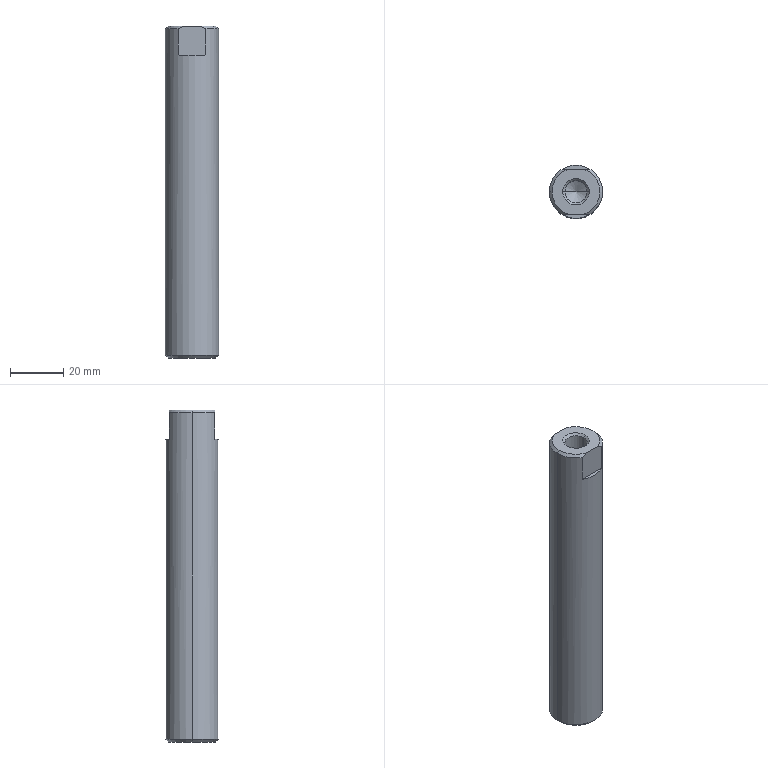Part | SolidWorks | features BaseBody 1 | 1 solid | 19 faces | box 20 x 20 x 125 mm | volume 37828 mm3 | cone 9 | plane 6 | cylinder 4 | commonest cylinder face diameters 8.376 x2 20 x2
STEP:
#1=CARTESIAN_POINT('',(10.,0.,-124.));
#2=VERTEX_POINT('',#1);
#3=CARTESIAN_POINT('',(-10.,0.,-124.));
#4=VERTEX_POINT('',#3);
#5=CARTESIAN_POINT('',(0.,0.,-124.));
#6=DIRECTION('',(0.,0.,1.));
#7=DIRECTION('',(1.,0.,0.));
#8=AXIS2_PLACEMENT_3D('',#5,#6,#7);
#9=CIRCLE('',#8,10.);
#10=EDGE_CURVE('',#2,#4,#9,.T.);
#11=ORIENTED_EDGE('',*,*,#10,.T.);
#12=CARTESIAN_POINT('',(-10.,0.,-1.));
#13=VERTEX_POINT('',#12);
#14=CARTESIAN_POINT('',(-10.,0.,-125.));
#15=DIRECTION('',(0.,0.,1.));
#16=VECTOR('',#15,1000.);
#17=LINE('',#14,#16);
#18=EDGE_CURVE('',#4,#13,#17,.T.);
#19=ORIENTED_EDGE('',*,*,#18,.T.);
#20=CARTESIAN_POINT('',(-5.268,8.5,-1.));
#21=VERTEX_POINT('',#20);
#22=CARTESIAN_POINT('',(0.,0.,-1.));
#23=DIRECTION('',(0.,0.,-1.));
#24=DIRECTION('',(1.,0.,0.));
#25=AXIS2_PLACEMENT_3D('',#22,#23,#24);
#26=CIRCLE('',#25,10.);
#27=EDGE_CURVE('',#13,#21,#26,.T.);
#28=ORIENTED_EDGE('',*,*,#27,.T.);
#29=CARTESIAN_POINT('',(-5.268,8.5,-11.));
#30=VERTEX_POINT('',#29);
#31=CARTESIAN_POINT('',(-5.268,8.5,-125.));
#32=DIRECTION('',(0.,0.,-1.));
#33=VECTOR('',#32,1000.);
#34=LINE('',#31,#33);
#35=EDGE_CURVE('',#21,#30,#34,.T.);
#36=ORIENTED_EDGE('',*,*,#35,.T.);
#37=CARTESIAN_POINT('',(5.268,8.5,-11.));
#38=VERTEX_POINT('',#37);
#39=CARTESIAN_POINT('',(0.,0.,-11.));
#40=DIRECTION('',(0.,0.,-1.));
#41=DIRECTION('',(1.,0.,0.));
#42=AXIS2_PLACEMENT_3D('',#39,#40,#41);
#43=CIRCLE('',#42,10.);
#44=EDGE_CURVE('',#30,#38,#43,.T.);
#45=ORIENTED_EDGE('',*,*,#44,.T.);
#46=CARTESIAN_POINT('',(5.268,8.5,-1.));
#47=VERTEX_POINT('',#46);
#48=CARTESIAN_POINT('',(5.268,8.5,-125.));
#49=DIRECTION('',(0.,0.,1.));
#50=VECTOR('',#49,1000.);
#51=LINE('',#48,#50);
#52=EDGE_CURVE('',#38,#47,#51,.T.);
#53=ORIENTED_EDGE('',*,*,#52,.T.);
#54=CARTESIAN_POINT('',(10.,0.,-1.));
#55=VERTEX_POINT('',#54);
#56=CARTESIAN_POINT('',(0.,0.,-1.));
#57=DIRECTION('',(0.,0.,-1.));
#58=DIRECTION('',(1.,0.,0.));
#59=AXIS2_PLACEMENT_3D('',#56,#57,#58);
#60=CIRCLE('',#59,10.);
#61=EDGE_CURVE('',#47,#55,#60,.T.);
#62=ORIENTED_EDGE('',*,*,#61,.T.);
#63=CARTESIAN_POINT('',(10.,0.,-125.));
#64=DIRECTION('',(0.,0.,1.));
#65=VECTOR('',#64,1000.);
#66=LINE('',#63,#65);
#67=EDGE_CURVE('',#2,#55,#66,.T.);
#68=ORIENTED_EDGE('',*,*,#67,.F.);
#69=EDGE_LOOP('',(#11,#19,#28,#36,#45,#53,#62,#68));
#70=FACE_OUTER_BOUND('',#69,.T.);
#71=CARTESIAN_POINT('',(0.,0.,-125.));
#72=DIRECTION('',(0.,0.,1.));
#73=DIRECTION('',(1.,0.,0.));
#74=AXIS2_PLACEMENT_3D('',#71,#72,#73);
#75=CYLINDRICAL_SURFACE('',#74,10.);
#76=ADVANCED_FACE('',(#70),#75,.T.);
#77=CARTESIAN_POINT('',(-2.958,-8.5,0.));
#78=VERTEX_POINT('',#77);
#79=CARTESIAN_POINT('',(-9.,0.,0.));
#80=VERTEX_POINT('',#79);
#81=CARTESIAN_POINT('',(0.,0.,0.));
#82=DIRECTION('',(0.,0.,-1.));
#83=DIRECTION('',(-1.,0.,0.));
#84=AXIS2_PLACEMENT_3D('',#81,#82,#83);
#85=CIRCLE('',#84,9.);
#86=EDGE_CURVE('',#78,#80,#85,.T.);
#87=ORIENTED_EDGE('',*,*,#86,.T.);
#88=CARTESIAN_POINT('',(-10.,0.,-1.));
#89=DIRECTION('',(-0.7071,0.,-0.7071));
#90=VECTOR('',#89,1000.);
#91=LINE('',#88,#90);
#92=EDGE_CURVE('',#80,#13,#91,.T.);
#93=ORIENTED_EDGE('',*,*,#92,.T.);
#94=CARTESIAN_POINT('',(-5.268,-8.5,-1.));
#95=VERTEX_POINT('',#94);
#96=CARTESIAN_POINT('',(0.,0.,-1.));
#97=DIRECTION('',(0.,0.,-1.));
#98=DIRECTION('',(1.,0.,0.));
#99=AXIS2_PLACEMENT_3D('',#96,#97,#98);
#100=CIRCLE('',#99,10.);
#101=EDGE_CURVE('',#95,#13,#100,.T.);
#102=ORIENTED_EDGE('',*,*,#101,.F.);
#103=CARTESIAN_POINT('',(-5.268,-8.5,-1.));
#104=CARTESIAN_POINT('',(-4.523,-8.5,-0.6078));
#105=CARTESIAN_POINT('',(-3.758,-8.5,-0.2631));
#106=CARTESIAN_POINT('',(-2.958,-8.5,0.));
#107=B_SPLINE_CURVE_WITH_KNOTS('',3,(#103,#104,#105,#106),.UNSPECIFIED.,.F.,.F.,(4,4),(0.,0.002517),.UNSPECIFIED.);
#108=EDGE_CURVE('',#95,#78,#107,.T.);
#109=ORIENTED_EDGE('',*,*,#108,.T.);
#110=EDGE_LOOP('',(#87,#93,#102,#109));
#111=FACE_OUTER_BOUND('',#110,.T.);
#112=CARTESIAN_POINT('',(0.,0.,-1.));
#113=DIRECTION('',(0.,0.,-1.));
#114=DIRECTION('',(-1.,0.,0.));
#115=AXIS2_PLACEMENT_3D('',#112,#113,#114);
#116=CONICAL_SURFACE('',#115,10.,0.7854);
#117=ADVANCED_FACE('',(#111),#116,.T.);
#118=CARTESIAN_POINT('',(9.,0.,-125.));
#119=VERTEX_POINT('',#118);
#120=CARTESIAN_POINT('',(-9.,0.,-125.));
#121=VERTEX_POINT('',#120);
#122=CARTESIAN_POINT('',(0.,0.,-125.));
#123=DIRECTION('',(0.,0.,1.));
#124=DIRECTION('',(1.,0.,0.));
#125=AXIS2_PLACEMENT_3D('',#122,#123,#124);
#126=CIRCLE('',#125,9.);
#127=EDGE_CURVE('',#119,#121,#126,.T.);
#128=ORIENTED_EDGE('',*,*,#127,.T.);
#129=CARTESIAN_POINT('',(-10.,0.,-124.));
#130=DIRECTION('',(-0.7071,0.,0.7071));
#131=VECTOR('',#130,1000.);
#132=LINE('',#129,#131);
#133=EDGE_CURVE('',#121,#4,#132,.T.);
#134=ORIENTED_EDGE('',*,*,#133,.T.);
#135=ORIENTED_EDGE('',*,*,#10,.F.);
#136=CARTESIAN_POINT('',(10.,0.,-124.));
#137=DIRECTION('',(0.7071,0.,0.7071));
#138=VECTOR('',#137,1000.);
#139=LINE('',#136,#138);
#140=EDGE_CURVE('',#119,#2,#139,.T.);
#141=ORIENTED_EDGE('',*,*,#140,.F.);
#142=EDGE_LOOP('',(#128,#134,#135,#141));
#143=FACE_OUTER_BOUND('',#142,.T.);
#144=CARTESIAN_POINT('',(0.,0.,-124.));
#145=DIRECTION('',(0.,0.,1.));
#146=DIRECTION('',(1.,0.,0.));
#147=AXIS2_PLACEMENT_3D('',#144,#145,#146);
#148=CONICAL_SURFACE('',#147,10.,0.7854);
#149=ADVANCED_FACE('',(#143),#148,.T.);
#150=CARTESIAN_POINT('',(-4.188,0.,-0.812));
#151=VERTEX_POINT('',#150);
#152=CARTESIAN_POINT('',(4.188,0.,-0.812));
#153=VERTEX_POINT('',#152);
#154=CARTESIAN_POINT('',(0.,0.,-0.812));
#155=DIRECTION('',(0.,0.,1.));
#156=DIRECTION('',(1.,0.,0.));
#157=AXIS2_PLACEMENT_3D('',#154,#155,#156);
#158=CIRCLE('',#157,4.188);
#159=EDGE_CURVE('',#151,#153,#158,.T.);
#160=ORIENTED_EDGE('',*,*,#159,.F.);
#161=CARTESIAN_POINT('',(-5.,0.,0.));
#162=VERTEX_POINT('',#161);
#163=CARTESIAN_POINT('',(-5.,0.,0.));
#164=DIRECTION('',(-0.7071,0.,0.7071));
#165=VECTOR('',#164,1000.);
#166=LINE('',#163,#165);
#167=EDGE_CURVE('',#151,#162,#166,.T.);
#168=ORIENTED_EDGE('',*,*,#167,.T.);
#169=CARTESIAN_POINT('',(5.,0.,0.));
#170=VERTEX_POINT('',#169);
#171=CARTESIAN_POINT('',(0.,0.,0.));
#172=DIRECTION('',(0.,0.,1.));
#173=DIRECTION('',(1.,0.,0.));
#174=AXIS2_PLACEMENT_3D('',#171,#172,#173);
#175=CIRCLE('',#174,5.);
#176=EDGE_CURVE('',#162,#170,#175,.T.);
#177=ORIENTED_EDGE('',*,*,#176,.T.);
#178=CARTESIAN_POINT('',(5.,0.,0.));
#179=DIRECTION('',(0.7071,0.,0.7071));
#180=VECTOR('',#179,1000.);
#181=LINE('',#178,#180);
#182=EDGE_CURVE('',#153,#170,#181,.T.);
#183=ORIENTED_EDGE('',*,*,#182,.F.);
#184=EDGE_LOOP('',(#160,#168,#177,#183));
#185=FACE_OUTER_BOUND('',#184,.T.);
#186=CARTESIAN_POINT('',(0.,0.,0.));
#187=DIRECTION('',(0.,0.,1.));
#188=DIRECTION('',(1.,0.,0.));
#189=AXIS2_PLACEMENT_3D('',#186,#187,#188);
#190=CONICAL_SURFACE('',#189,5.,0.7854);
#191=ADVANCED_FACE('',(#185),#190,.F.);
#192=CARTESIAN_POINT('',(-4.188,0.,-20.));
#193=VERTEX_POINT('',#192);
#194=CARTESIAN_POINT('',(4.188,0.,-20.));
#195=VERTEX_POINT('',#194);
#196=CARTESIAN_POINT('',(0.,0.,-20.));
#197=DIRECTION('',(0.,0.,1.));
#198=DIRECTION('',(1.,0.,0.));
#199=AXIS2_PLACEMENT_3D('',#196,#197,#198);
#200=CIRCLE('',#199,4.188);
#201=EDGE_CURVE('',#193,#195,#200,.T.);
#202=ORIENTED_EDGE('',*,*,#201,.F.);
#203=CARTESIAN_POINT('',(-4.188,0.,-22.418));
#204=DIRECTION('',(0.,0.,1.));
#205=VECTOR('',#204,1000.);
#206=LINE('',#203,#205);
#207=EDGE_CURVE('',#193,#151,#206,.T.);
#208=ORIENTED_EDGE('',*,*,#207,.T.);
#209=ORIENTED_EDGE('',*,*,#159,.T.);
#210=CARTESIAN_POINT('',(4.188,0.,-22.418));
#211=DIRECTION('',(0.,0.,1.));
#212=VECTOR('',#211,1000.);
#213=LINE('',#210,#212);
#214=EDGE_CURVE('',#195,#153,#213,.T.);
#215=ORIENTED_EDGE('',*,*,#214,.F.);
#216=EDGE_LOOP('',(#202,#208,#209,#215));
#217=FACE_OUTER_BOUND('',#216,.T.);
#218=CARTESIAN_POINT('',(0.,0.,-22.418));
#219=DIRECTION('',(0.,0.,1.));
#220=DIRECTION('',(1.,0.,0.));
#221=AXIS2_PLACEMENT_3D('',#218,#219,#220);
#222=CYLINDRICAL_SURFACE('',#221,4.188);
#223=ADVANCED_FACE('',(#217),#222,.F.);
#224=CARTESIAN_POINT('',(0.,0.,-22.418));
#225=VERTEX_POINT('',#224);
#226=CARTESIAN_POINT('',(4.188,0.,-20.));
#227=DIRECTION('',(0.866,0.,0.5));
#228=VECTOR('',#227,1000.);
#229=LINE('',#226,#228);
#230=EDGE_CURVE('',#225,#195,#229,.T.);
#231=ORIENTED_EDGE('',*,*,#230,.F.);
#232=CARTESIAN_POINT('',(-4.188,0.,-20.));
#233=DIRECTION('',(-0.866,0.,0.5));
#234=VECTOR('',#233,1000.);
#235=LINE('',#232,#234);
#236=EDGE_CURVE('',#225,#193,#235,.T.);
#237=ORIENTED_EDGE('',*,*,#236,.T.);
#238=ORIENTED_EDGE('',*,*,#201,.T.);
#239=EDGE_LOOP('',(#231,#237,#238));
#240=FACE_OUTER_BOUND('',#239,.T.);
#241=CARTESIAN_POINT('',(0.,0.,-20.));
#242=DIRECTION('',(0.,0.,1.));
#243=DIRECTION('',(1.,0.,0.));
#244=AXIS2_PLACEMENT_3D('',#241,#242,#243);
#245=CONICAL_SURFACE('',#244,4.188,1.047);
#246=ADVANCED_FACE('',(#240),#245,.F.);
#247=ORIENTED_EDGE('',*,*,#18,.F.);
#248=CARTESIAN_POINT('',(0.,0.,-124.));
#249=DIRECTION('',(0.,0.,1.));
#250=DIRECTION('',(1.,0.,0.));
#251=AXIS2_PLACEMENT_3D('',#248,#249,#250);
#252=CIRCLE('',#251,10.);
#253=EDGE_CURVE('',#4,#2,#252,.T.);
#254=ORIENTED_EDGE('',*,*,#253,.T.);
#255=ORIENTED_EDGE('',*,*,#67,.T.);
#256=CARTESIAN_POINT('',(5.268,-8.5,-1.));
#257=VERTEX_POINT('',#256);
#258=CARTESIAN_POINT('',(0.,0.,-1.));
#259=DIRECTION('',(0.,0.,-1.));
#260=DIRECTION('',(1.,0.,0.));
#261=AXIS2_PLACEMENT_3D('',#258,#259,#260);
#262=CIRCLE('',#261,10.);
#263=EDGE_CURVE('',#55,#257,#262,.T.);
#264=ORIENTED_EDGE('',*,*,#263,.T.);
#265=CARTESIAN_POINT('',(5.268,-8.5,-11.));
#266=VERTEX_POINT('',#265);
#267=CARTESIAN_POINT('',(5.268,-8.5,-125.));
#268=DIRECTION('',(0.,0.,-1.));
#269=VECTOR('',#268,1000.);
#270=LINE('',#267,#269);
#271=EDGE_CURVE('',#257,#266,#270,.T.);
#272=ORIENTED_EDGE('',*,*,#271,.T.);
#273=CARTESIAN_POINT('',(-5.268,-8.5,-11.));
#274=VERTEX_POINT('',#273);
#275=CARTESIAN_POINT('',(0.,0.,-11.));
#276=DIRECTION('',(0.,0.,-1.));
#277=DIRECTION('',(1.,0.,0.));
#278=AXIS2_PLACEMENT_3D('',#275,#276,#277);
#279=CIRCLE('',#278,10.);
#280=EDGE_CURVE('',#266,#274,#279,.T.);
#281=ORIENTED_EDGE('',*,*,#280,.T.);
#282=CARTESIAN_POINT('',(-5.268,-8.5,-125.));
#283=DIRECTION('',(0.,0.,1.));
#284=VECTOR('',#283,1000.);
#285=LINE('',#282,#284);
#286=EDGE_CURVE('',#274,#95,#285,.T.);
#287=ORIENTED_EDGE('',*,*,#286,.T.);
#288=ORIENTED_EDGE('',*,*,#101,.T.);
#289=EDGE_LOOP('',(#247,#254,#255,#264,#272,#281,#287,#288));
#290=FACE_OUTER_BOUND('',#289,.T.);
#291=CARTESIAN_POINT('',(0.,0.,-125.));
#292=DIRECTION('',(0.,0.,1.));
#293=DIRECTION('',(1.,0.,0.));
#294=AXIS2_PLACEMENT_3D('',#291,#292,#293);
#295=CYLINDRICAL_SURFACE('',#294,10.);
#296=ADVANCED_FACE('',(#290),#295,.T.);
#297=CARTESIAN_POINT('',(5.268,8.5,-11.));
#298=DIRECTION('',(-1.,0.,0.));
#299=VECTOR('',#298,1000.);
#300=LINE('',#297,#299);
#301=EDGE_CURVE('',#38,#30,#300,.T.);
#302=ORIENTED_EDGE('',*,*,#301,.T.);
#303=ORIENTED_EDGE('',*,*,#35,.F.);
#304=CARTESIAN_POINT('',(-2.958,8.5,0.));
#305=VERTEX_POINT('',#304);
#306=CARTESIAN_POINT('',(-5.268,8.5,-1.));
#307=CARTESIAN_POINT('',(-4.523,8.5,-0.6078));
#308=CARTESIAN_POINT('',(-3.758,8.5,-0.2631));
#309=CARTESIAN_POINT('',(-2.958,8.5,0.));
#310=B_SPLINE_CURVE_WITH_KNOTS('',3,(#306,#307,#308,#309),.UNSPECIFIED.,.F.,.F.,(4,4),(0.,0.002517),.UNSPECIFIED.);
#311=EDGE_CURVE('',#21,#305,#310,.T.);
#312=ORIENTED_EDGE('',*,*,#311,.T.);
#313=CARTESIAN_POINT('',(2.958,8.5,0.));
#314=VERTEX_POINT('',#313);
#315=CARTESIAN_POINT('',(5.268,8.5,0.));
#316=DIRECTION('',(1.,0.,0.));
#317=VECTOR('',#316,1000.);
#318=LINE('',#315,#317);
#319=EDGE_CURVE('',#305,#314,#318,.T.);
#320=ORIENTED_EDGE('',*,*,#319,.T.);
#321=CARTESIAN_POINT('',(2.958,8.5,0.));
#322=CARTESIAN_POINT('',(3.758,8.5,-0.2631));
#323=CARTESIAN_POINT('',(4.523,8.5,-0.6078));
#324=CARTESIAN_POINT('',(5.268,8.5,-1.));
#325=B_SPLINE_CURVE_WITH_KNOTS('',3,(#321,#322,#323,#324),.UNSPECIFIED.,.F.,.F.,(4,4),(0.,0.002517),.UNSPECIFIED.);
#326=EDGE_CURVE('',#314,#47,#325,.T.);
#327=ORIENTED_EDGE('',*,*,#326,.T.);
#328=ORIENTED_EDGE('',*,*,#52,.F.);
#329=EDGE_LOOP('',(#302,#303,#312,#320,#327,#328));
#330=FACE_OUTER_BOUND('',#329,.T.);
#331=CARTESIAN_POINT('',(5.268,8.5,-11.));
#332=DIRECTION('',(0.,1.,0.));
#333=DIRECTION('',(0.,0.,1.));
#334=AXIS2_PLACEMENT_3D('',#331,#332,#333);
#335=PLANE('',#334);
#336=ADVANCED_FACE('',(#330),#335,.T.);
#337=ORIENTED_EDGE('',*,*,#92,.F.);
#338=CARTESIAN_POINT('',(0.,0.,0.));
#339=DIRECTION('',(0.,0.,-1.));
#340=DIRECTION('',(-1.,0.,0.));
#341=AXIS2_PLACEMENT_3D('',#338,#339,#340);
#342=CIRCLE('',#341,9.);
#343=EDGE_CURVE('',#80,#305,#342,.T.);
#344=ORIENTED_EDGE('',*,*,#343,.T.);
#345=ORIENTED_EDGE('',*,*,#311,.F.);
#346=ORIENTED_EDGE('',*,*,#27,.F.);
#347=EDGE_LOOP('',(#337,#344,#345,#346));
#348=FACE_OUTER_BOUND('',#347,.T.);
#349=CARTESIAN_POINT('',(0.,0.,-1.));
#350=DIRECTION('',(0.,0.,-1.));
#351=DIRECTION('',(-1.,0.,0.));
#352=AXIS2_PLACEMENT_3D('',#349,#350,#351);
#353=CONICAL_SURFACE('',#352,10.,0.7854);
#354=ADVANCED_FACE('',(#348),#353,.T.);
#355=CARTESIAN_POINT('',(-5.268,-8.5,-11.));
#356=DIRECTION('',(1.,0.,0.));
#357=VECTOR('',#356,1000.);
#358=LINE('',#355,#357);
#359=EDGE_CURVE('',#274,#266,#358,.T.);
#360=ORIENTED_EDGE('',*,*,#359,.T.);
#361=ORIENTED_EDGE('',*,*,#271,.F.);
#362=CARTESIAN_POINT('',(2.958,-8.5,0.));
#363=VERTEX_POINT('',#362);
#364=CARTESIAN_POINT('',(5.268,-8.5,-1.));
#365=CARTESIAN_POINT('',(4.523,-8.5,-0.6078));
#366=CARTESIAN_POINT('',(3.758,-8.5,-0.2631));
#367=CARTESIAN_POINT('',(2.958,-8.5,0.));
#368=B_SPLINE_CURVE_WITH_KNOTS('',3,(#364,#365,#366,#367),.UNSPECIFIED.,.F.,.F.,(4,4),(0.,0.002517),.UNSPECIFIED.);
#369=EDGE_CURVE('',#257,#363,#368,.T.);
#370=ORIENTED_EDGE('',*,*,#369,.T.);
#371=CARTESIAN_POINT('',(-5.268,-8.5,0.));
#372=DIRECTION('',(-1.,0.,0.));
#373=VECTOR('',#372,1000.);
#374=LINE('',#371,#373);
#375=EDGE_CURVE('',#363,#78,#374,.T.);
#376=ORIENTED_EDGE('',*,*,#375,.T.);
#377=ORIENTED_EDGE('',*,*,#108,.F.);
#378=ORIENTED_EDGE('',*,*,#286,.F.);
#379=EDGE_LOOP('',(#360,#361,#370,#376,#377,#378));
#380=FACE_OUTER_BOUND('',#379,.T.);
#381=CARTESIAN_POINT('',(-5.268,-8.5,-11.));
#382=DIRECTION('',(0.,-1.,0.));
#383=DIRECTION('',(0.,0.,-1.));
#384=AXIS2_PLACEMENT_3D('',#381,#382,#383);
#385=PLANE('',#384);
#386=ADVANCED_FACE('',(#380),#385,.T.);
#387=ORIENTED_EDGE('',*,*,#280,.F.);
#388=ORIENTED_EDGE('',*,*,#359,.F.);
#389=EDGE_LOOP('',(#387,#388));
#390=FACE_OUTER_BOUND('',#389,.T.);
#391=CARTESIAN_POINT('',(0.,0.,-11.));
#392=DIRECTION('',(0.,0.,1.));
#393=DIRECTION('',(1.,0.,0.));
#394=AXIS2_PLACEMENT_3D('',#391,#392,#393);
#395=PLANE('',#394);
#396=ADVANCED_FACE('',(#390),#395,.T.);
#397=ORIENTED_EDGE('',*,*,#369,.F.);
#398=ORIENTED_EDGE('',*,*,#263,.F.);
#399=ORIENTED_EDGE('',*,*,#61,.F.);
#400=ORIENTED_EDGE('',*,*,#326,.F.);
#401=CARTESIAN_POINT('',(0.,0.,0.));
#402=DIRECTION('',(0.,0.,-1.));
#403=DIRECTION('',(-1.,0.,0.));
#404=AXIS2_PLACEMENT_3D('',#401,#402,#403);
#405=CIRCLE('',#404,9.);
#406=EDGE_CURVE('',#314,#363,#405,.T.);
#407=ORIENTED_EDGE('',*,*,#406,.T.);
#408=EDGE_LOOP('',(#397,#398,#399,#400,#407));
#409=FACE_OUTER_BOUND('',#408,.T.);
#410=CARTESIAN_POINT('',(0.,0.,-1.));
#411=DIRECTION('',(0.,0.,-1.));
#412=DIRECTION('',(-1.,0.,0.));
#413=AXIS2_PLACEMENT_3D('',#410,#411,#412);
#414=CONICAL_SURFACE('',#413,10.,0.7854);
#415=ADVANCED_FACE('',(#409),#414,.T.);
#416=ORIENTED_EDGE('',*,*,#44,.F.);
#417=ORIENTED_EDGE('',*,*,#301,.F.);
#418=EDGE_LOOP('',(#416,#417));
#419=FACE_OUTER_BOUND('',#418,.T.);
#420=CARTESIAN_POINT('',(0.,0.,-11.));
#421=DIRECTION('',(0.,0.,1.));
#422=DIRECTION('',(1.,0.,0.));
#423=AXIS2_PLACEMENT_3D('',#420,#421,#422);
#424=PLANE('',#423);
#425=ADVANCED_FACE('',(#419),#424,.T.);
#426=ORIENTED_EDGE('',*,*,#133,.F.);
#427=CARTESIAN_POINT('',(0.,0.,-125.));
#428=DIRECTION('',(0.,0.,1.));
#429=DIRECTION('',(1.,0.,0.));
#430=AXIS2_PLACEMENT_3D('',#427,#428,#429);
#431=CIRCLE('',#430,9.);
#432=EDGE_CURVE('',#121,#119,#431,.T.);
#433=ORIENTED_EDGE('',*,*,#432,.T.);
#434=ORIENTED_EDGE('',*,*,#140,.T.);
#435=ORIENTED_EDGE('',*,*,#253,.F.);
#436=EDGE_LOOP('',(#426,#433,#434,#435));
#437=FACE_OUTER_BOUND('',#436,.T.);
#438=CARTESIAN_POINT('',(0.,0.,-124.));
#439=DIRECTION('',(0.,0.,1.));
#440=DIRECTION('',(1.,0.,0.));
#441=AXIS2_PLACEMENT_3D('',#438,#439,#440);
#442=CONICAL_SURFACE('',#441,10.,0.7854);
#443=ADVANCED_FACE('',(#437),#442,.T.);
#444=CARTESIAN_POINT('',(0.,0.,0.));
#445=DIRECTION('',(0.,0.,1.));
#446=DIRECTION('',(1.,0.,0.));
#447=AXIS2_PLACEMENT_3D('',#444,#445,#446);
#448=CIRCLE('',#447,5.);
#449=EDGE_CURVE('',#170,#162,#448,.T.);
#450=ORIENTED_EDGE('',*,*,#449,.F.);
#451=ORIENTED_EDGE('',*,*,#176,.F.);
#452=EDGE_LOOP('',(#450,#451));
#453=FACE_BOUND('',#452,.T.);
#454=ORIENTED_EDGE('',*,*,#375,.F.);
#455=ORIENTED_EDGE('',*,*,#406,.F.);
#456=ORIENTED_EDGE('',*,*,#319,.F.);
#457=ORIENTED_EDGE('',*,*,#343,.F.);
#458=ORIENTED_EDGE('',*,*,#86,.F.);
#459=EDGE_LOOP('',(#454,#455,#456,#457,#458));
#460=FACE_OUTER_BOUND('',#459,.T.);
#461=CARTESIAN_POINT('',(0.,0.,0.));
#462=DIRECTION('',(0.,0.,-1.));
#463=DIRECTION('',(-1.,0.,0.));
#464=AXIS2_PLACEMENT_3D('',#461,#462,#463);
#465=PLANE('',#464);
#466=ADVANCED_FACE('',(#453,#460),#465,.F.);
#467=ORIENTED_EDGE('',*,*,#127,.F.);
#468=ORIENTED_EDGE('',*,*,#432,.F.);
#469=EDGE_LOOP('',(#467,#468));
#470=FACE_OUTER_BOUND('',#469,.T.);
#471=CARTESIAN_POINT('',(-9.,0.,-125.));
#472=DIRECTION('',(0.,0.,1.));
#473=DIRECTION('',(1.,0.,0.));
#474=AXIS2_PLACEMENT_3D('',#471,#472,#473);
#475=PLANE('',#474);
#476=ADVANCED_FACE('',(#470),#475,.F.);
#477=ORIENTED_EDGE('',*,*,#167,.F.);
#478=CARTESIAN_POINT('',(0.,0.,-0.812));
#479=DIRECTION('',(0.,0.,1.));
#480=DIRECTION('',(1.,0.,0.));
#481=AXIS2_PLACEMENT_3D('',#478,#479,#480);
#482=CIRCLE('',#481,4.188);
#483=EDGE_CURVE('',#153,#151,#482,.T.);
#484=ORIENTED_EDGE('',*,*,#483,.F.);
#485=ORIENTED_EDGE('',*,*,#182,.T.);
#486=ORIENTED_EDGE('',*,*,#449,.T.);
#487=EDGE_LOOP('',(#477,#484,#485,#486));
#488=FACE_OUTER_BOUND('',#487,.T.);
#489=CARTESIAN_POINT('',(0.,0.,0.));
#490=DIRECTION('',(0.,0.,1.));
#491=DIRECTION('',(1.,0.,0.));
#492=AXIS2_PLACEMENT_3D('',#489,#490,#491);
#493=CONICAL_SURFACE('',#492,5.,0.7854);
#494=ADVANCED_FACE('',(#488),#493,.F.);
#495=ORIENTED_EDGE('',*,*,#207,.F.);
#496=CARTESIAN_POINT('',(0.,0.,-20.));
#497=DIRECTION('',(0.,0.,1.));
#498=DIRECTION('',(1.,0.,0.));
#499=AXIS2_PLACEMENT_3D('',#496,#497,#498);
#500=CIRCLE('',#499,4.188);
#501=EDGE_CURVE('',#195,#193,#500,.T.);
#502=ORIENTED_EDGE('',*,*,#501,.F.);
#503=ORIENTED_EDGE('',*,*,#214,.T.);
#504=ORIENTED_EDGE('',*,*,#483,.T.);
#505=EDGE_LOOP('',(#495,#502,#503,#504));
#506=FACE_OUTER_BOUND('',#505,.T.);
#507=CARTESIAN_POINT('',(0.,0.,-22.418));
#508=DIRECTION('',(0.,0.,1.));
#509=DIRECTION('',(1.,0.,0.));
#510=AXIS2_PLACEMENT_3D('',#507,#508,#509);
#511=CYLINDRICAL_SURFACE('',#510,4.188);
#512=ADVANCED_FACE('',(#506),#511,.F.);
#513=ORIENTED_EDGE('',*,*,#236,.F.);
#514=ORIENTED_EDGE('',*,*,#230,.T.);
#515=ORIENTED_EDGE('',*,*,#501,.T.);
#516=EDGE_LOOP('',(#513,#514,#515));
#517=FACE_OUTER_BOUND('',#516,.T.);
#518=CARTESIAN_POINT('',(0.,0.,-20.));
#519=DIRECTION('',(0.,0.,1.));
#520=DIRECTION('',(1.,0.,0.));
#521=AXIS2_PLACEMENT_3D('',#518,#519,#520);
#522=CONICAL_SURFACE('',#521,4.188,1.047);
#523=ADVANCED_FACE('',(#517),#522,.F.);
#524=CLOSED_SHELL('',(#76,#117,#149,#191,#223,#246,#296,#336,#354,#386,#396,#415,#425,#443,#466,#476,#494,#512,#523));
#525=MANIFOLD_SOLID_BREP('',#524);
#526=CARTESIAN_POINT('',(0.,0.,0.));
#527=DIRECTION('',(0.,0.,1.));
#528=DIRECTION('',(1.,0.,0.));
#529=AXIS2_PLACEMENT_3D('',#526,#527,#528);
#530=(LENGTH_UNIT()NAMED_UNIT(*)SI_UNIT(.MILLI.,.METRE.));
#531=UNCERTAINTY_MEASURE_WITH_UNIT(LENGTH_MEASURE(0.00001),#530,'','');
#532=(NAMED_UNIT(*)PLANE_ANGLE_UNIT()SI_UNIT($,.RADIAN.));
#533=(NAMED_UNIT(*)SI_UNIT($,.STERADIAN.)SOLID_ANGLE_UNIT());
#534=(GEOMETRIC_REPRESENTATION_CONTEXT(3)GLOBAL_UNCERTAINTY_ASSIGNED_CONTEXT((#531))GLOBAL_UNIT_ASSIGNED_CONTEXT((#530,#532,#533))REPRESENTATION_CONTEXT('',''));
#535=ADVANCED_BREP_SHAPE_REPRESENTATION('',(#525,#529),#534);